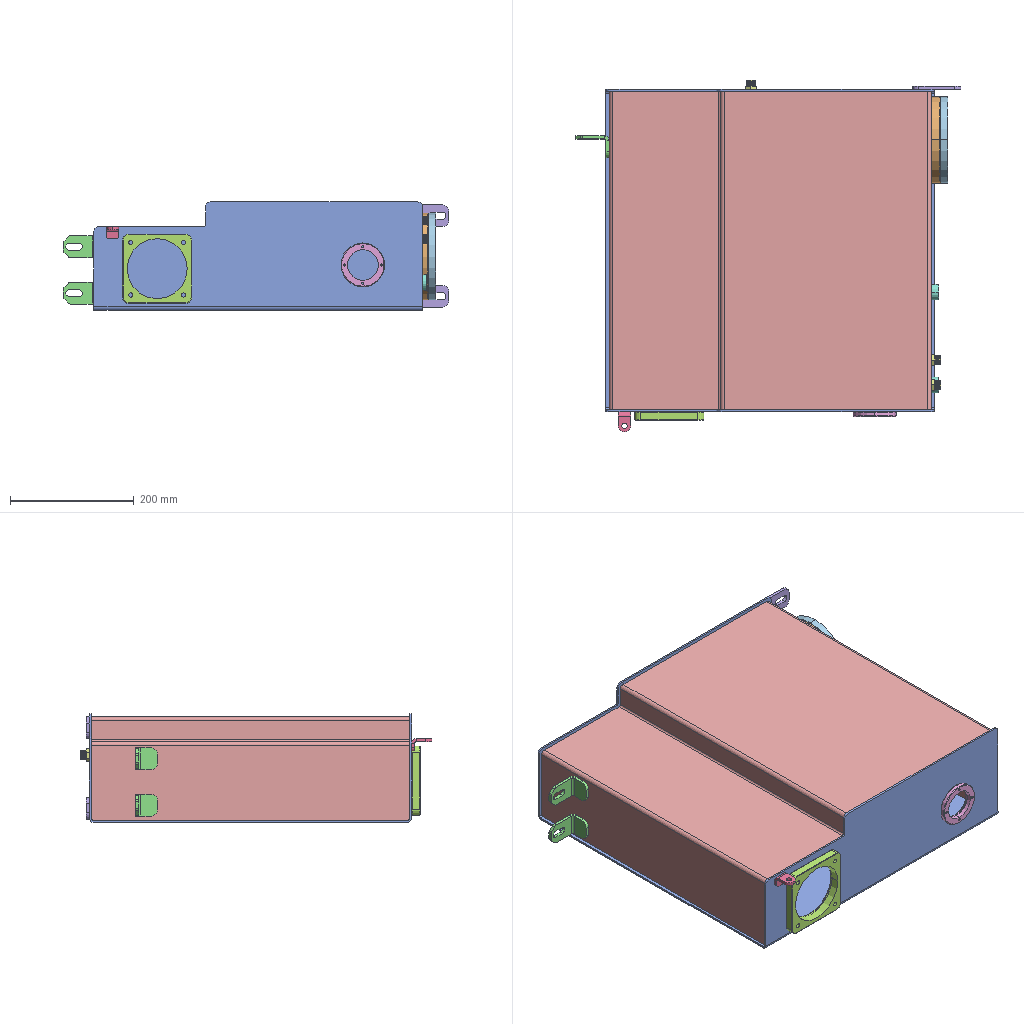Assembly | SolidWorks | 11 different items | 16 placed | box 623 x 568 x 175 mm
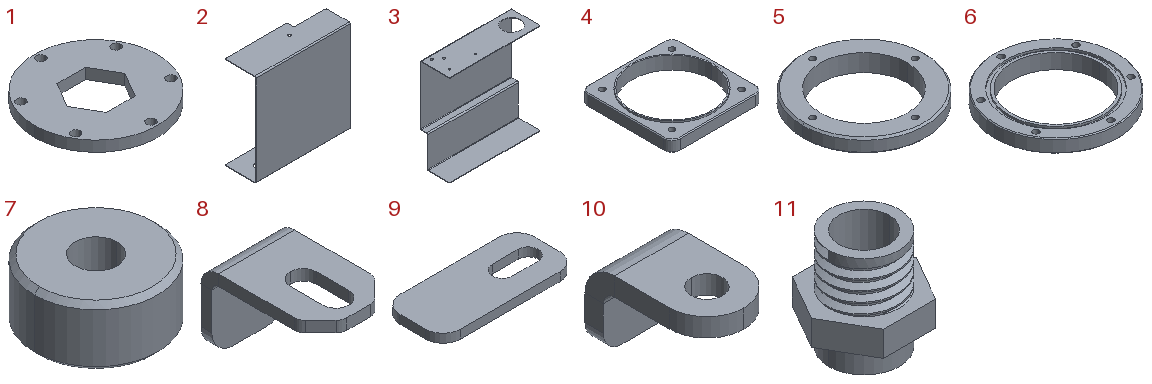Parts list (item | quantity | size | volume | features):
1 | x1 | 140 x 140 x 12 mm | 145896 mm3 | features Extrusion 1
2 | x1 | 530 x 175 x 520 mm | 1293540 mm3 | features Fillet 2, ICE 2, FlatPattern 1, SMBaseFlange 1, SheetMetal 1
3 | x1 | 514 x 167 x 520 mm | 1269270 mm3 | features Fillet 1, FlatPattern 1, ICE 1, SMBaseFlange 1, SheetMetal 1
4 | x1 | 112 x 112 x 16 mm | 69423 mm3 | features ICE 2, Chamfer 1, Extrusion 1, HoleWzd 1
5 | x1 | 71 x 71 x 10 mm | 15956 mm3 | features ICE 2, Chamfer 1, Extrusion 1, HoleWzd 1
6 | x1 | 140 x 140 x 17 mm | 108486 mm3 | features ICE 3, Chamfer 1, Extrusion 1, HoleWzd 1
7 | x2 | 25 x 25 x 12 mm | 5133 mm3 | features Chamfer 1, Extrusion 1, HoleWzd 1
8 | x2 | 35 x 55 x 35 mm | 12305 mm3 | features Fillet 2, Chamfer 1, FlatPattern 1, ICE 1, SMBaseFlange 1, SheetMetal 1
9 | x2 | 78 x 35 x 5 mm | 11789 mm3 | features Fillet 1, FlatPattern 1, SMBaseFlange 1, SheetMetal 1
10 | x1 | 20 x 33 x 20 mm | 4012 mm3 | features Fillet 2, FlatPattern 1, ICE 1, SMBaseFlange 1, SheetMetal 1
11 | x3 | 20.785 x 18 x 20 mm | 1890 mm3 | features ICE 2, Extrusion 1, SweepThread 1
Mates (type | each side: item.copy, entity, surface, feature):
Coincident | 3.1 face plane Base-Flange1 | 2.1 face plane Base-Flange1 | 2 times
DistanceDim | 3.1 face plane Base-Flange1 | 2.1 face plane Base-Flange1
Concentric | 2.1 face cylinder Cut-Extrude1 | 4.1 face cylinder Cut-Extrude2
Coincident | 2.1 face plane Base-Flange1 | 4.1 face plane Cut-Extrude2
Parallel | 2.1 face plane Base-Flange1 | 4.1 face plane Boss-Extrude1
Concentric | 2.1 face cylinder Cut-Extrude1 | 5.1 face cylinder Boss-Extrude1
Coincident | 2.1 face plane Base-Flange1 | 5.1 face plane Cut-Extrude2
Parallel | 5.1 plane | assembly plane
Coincident | 3.1 face plane Base-Flange1 | 7.1 face plane Boss-Extrude1
Concentric | 3.1 face cylinder Cut-Extrude1 | 7.1 face cylinder Boss-Extrude1
Coincident | 3.1 face plane Base-Flange1 | 7.2 face plane Boss-Extrude1
Concentric | 3.1 face cylinder Cut-Extrude1 | 7.2 face cylinder Boss-Extrude1
Coincident | 3.1 face plane Base-Flange1 | 6.1 face plane Cut-Extrude2
Concentric | 3.1 face cylinder Cut-Extrude1 | 6.1 face cylinder Boss-Extrude1
Coincident | 2.1 face plane Base-Flange1 | 9.1 face plane Base-Flange1
DistanceDim | 2.1 edge | 9.1 face plane Base-Flange1
DistanceDim | 2.1 face plane Base-Flange1 | 9.1 face plane Base-Flange1
Coincident | 2.1 face plane Base-Flange1 | 9.2 face plane Base-Flange1
DistanceDim | 9.2 face plane Base-Flange1 | 2.1 face plane Base-Flange1 | 2 times
Coincident | 3.1 face plane Base-Flange1 | 8.1 face plane Base-Flange1
DistanceDim | 8.1 face plane Base-Flange1 | 3.1 face plane Base-Flange1
DistanceDim | 8.1 face plane Base-Flange1 | 2.1 face plane Base-Flange1
Coincident | 3.1 face plane Base-Flange1 | 8.2 face plane Base-Flange1
DistanceDim | 2.1 face plane Base-Flange1 | 8.2 face plane Base-Flange1 | 2 times
Coincident | 2.1 face plane Base-Flange1 | 10.1 face plane Base-Flange1
Coincident | 2.1 face plane Cut-Extrude1 | 10.1 face plane Base-Flange1
DistanceDim | 2.1 face plane Base-Flange1 | 10.1 face plane Base-Flange1
Coincident | 6.1 face plane Boss-Extrude1 | 1.1 face plane Boss-Extrude1
Concentric | 6.1 face cylinder M8 Tapped Hole1 | 1.1 face cylinder Boss-Extrude1 | 2 times
Coincident | 3.1 face plane Base-Flange1 | 11.1 face plane Cut-Extrude2
Concentric | 3.1 face cylinder Cut-Extrude1 | 11.1 face cylinder Boss-Extrude1
Parallel | 2.1 face plane Base-Flange1 | 11.1 face plane Boss-Extrude1
Coincident | 3.1 face plane Base-Flange1 | 11.2 face plane Cut-Extrude2
Concentric | 3.1 face cylinder Cut-Extrude1 | 11.2 face cylinder Boss-Extrude1
Parallel | 2.1 face plane Base-Flange1 | 11.2 face plane Boss-Extrude1
Coincident | 2.1 face plane Base-Flange1 | 11.3 face plane Cut-Extrude2
Concentric | 2.1 face cylinder Cut-Extrude2 | 11.3 face cylinder Boss-Extrude1